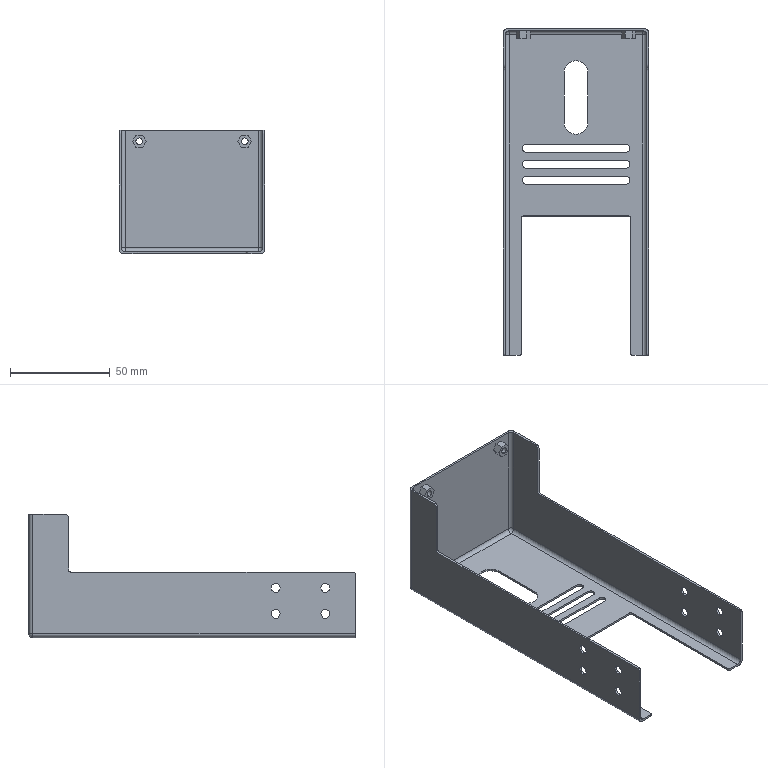Part | STEP file | 11-FG-B03411 | 1 solid | 95 faces | box 73 x 164 x 62 mm | volume 23088 mm3 | cylinder 51 | plane 40 | sphere 4 | commonest cylinder face diameters 4 x21 4.5 x16 2 x8 3.3 x4 12 x2